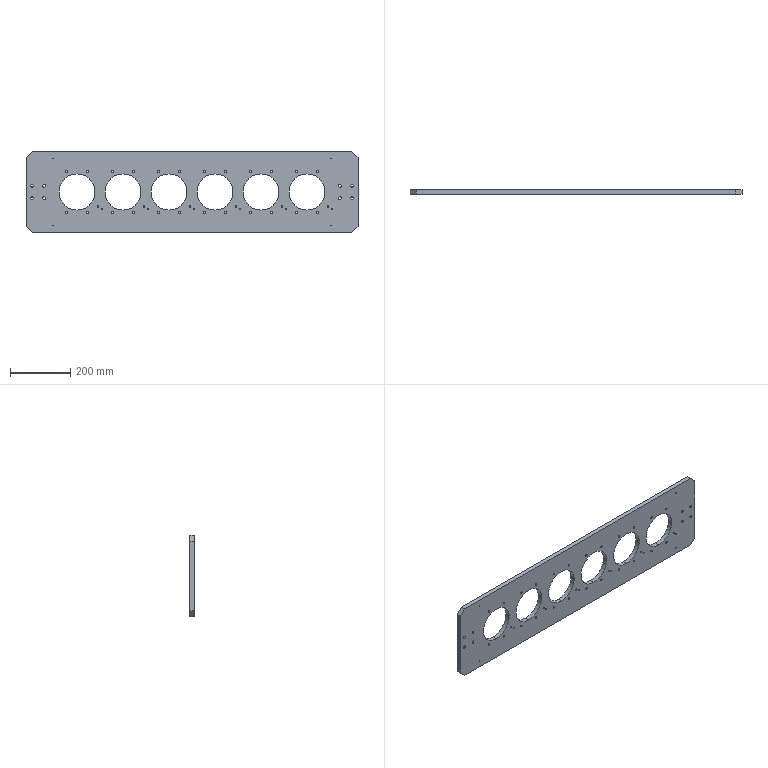Part | SolidWorks | features BaseBody 1 | 1 solid | 310 faces | box 1100 x 15 x 270 mm | volume 3383185 mm3 | cylinder 220 | cone 48 | plane 42 | commonest cylinder face diameters 2.5 x48 6.6 x48 11 x48 4.2 x24 9 x16 15 x16